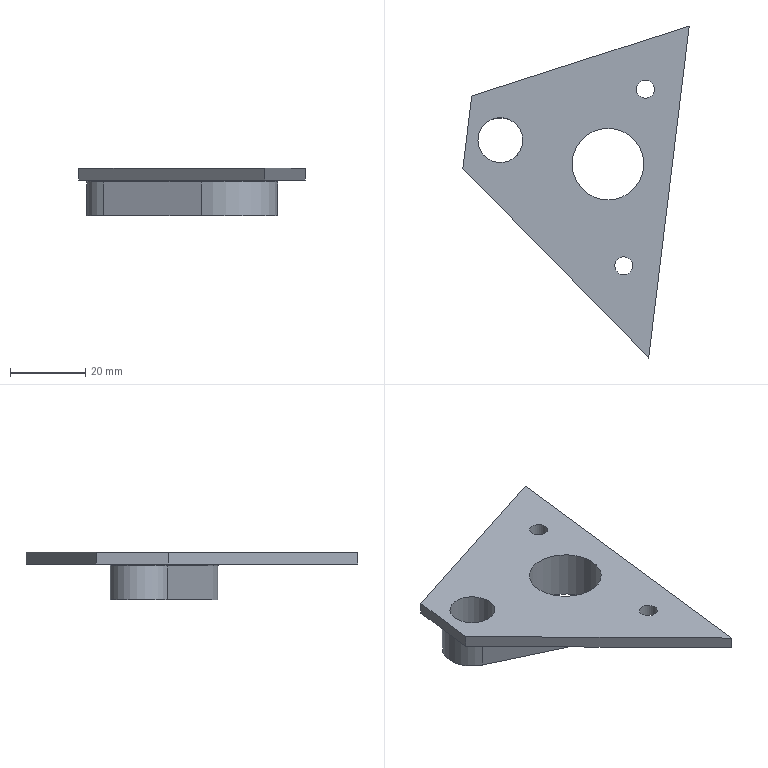Part | NX | features MG0301 nose pivot 24(left) 2 | 1 solid | 19 faces | box 60.073 x 88.114 x 12.7 mm | volume 14652 mm3 | plane 9 | cylinder 8 | torus 2 | commonest cylinder face diameters 1.016 x2 4.763 x2 11.906 x1 15.875 x1 19.05 x1 28.575 x1
STEP:
#1=CARTESIAN_POINT('',(-317.5,-112.204,-9.525));
#2=VERTEX_POINT('',#1);
#3=CARTESIAN_POINT('',(-346.075,-112.204,-9.525));
#4=VERTEX_POINT('',#3);
#5=CARTESIAN_POINT('',(-353.678,-112.204,-9.525));
#6=DIRECTION('',(-1.,0.,0.));
#7=VECTOR('',#6,1000.);
#8=LINE('',#5,#7);
#9=EDGE_CURVE('',#2,#4,#8,.T.);
#10=ORIENTED_EDGE('',*,*,#9,.T.);
#11=CARTESIAN_POINT('',(-349.652,-128.301,-9.525));
#12=VERTEX_POINT('',#11);
#13=CARTESIAN_POINT('',(-346.075,-120.65,-9.525));
#14=DIRECTION('',(0.,0.,1.));
#15=DIRECTION('',(1.,0.,0.));
#16=AXIS2_PLACEMENT_3D('',#13,#14,#15);
#17=CIRCLE('',#16,8.445);
#18=EDGE_CURVE('',#4,#12,#17,.T.);
#19=ORIENTED_EDGE('',*,*,#18,.T.);
#20=CARTESIAN_POINT('',(-323.766,-140.403,-9.525));
#21=VERTEX_POINT('',#20);
#22=CARTESIAN_POINT('',(-360.395,-123.278,-9.525));
#23=DIRECTION('',(0.9059,-0.4235,0.));
#24=VECTOR('',#23,1000.);
#25=LINE('',#22,#24);
#26=EDGE_CURVE('',#12,#21,#25,.T.);
#27=ORIENTED_EDGE('',*,*,#26,.T.);
#28=CARTESIAN_POINT('',(-317.5,-127.,-9.525));
#29=DIRECTION('',(0.,0.,1.));
#30=DIRECTION('',(1.,0.,0.));
#31=AXIS2_PLACEMENT_3D('',#28,#29,#30);
#32=CIRCLE('',#31,14.796);
#33=EDGE_CURVE('',#21,#2,#32,.T.);
#34=ORIENTED_EDGE('',*,*,#33,.T.);
#35=EDGE_LOOP('',(#10,#19,#27,#34));
#36=FACE_BOUND('',#35,.T.);
#37=CARTESIAN_POINT('',(-315.677,-153.957,-9.525));
#38=VERTEX_POINT('',#37);
#39=CARTESIAN_POINT('',(-313.296,-153.957,-9.525));
#40=DIRECTION('',(0.,0.,-1.));
#41=DIRECTION('',(-1.,0.,0.));
#42=AXIS2_PLACEMENT_3D('',#39,#40,#41);
#43=CIRCLE('',#42,2.381);
#44=EDGE_CURVE('',#38,#38,#43,.T.);
#45=ORIENTED_EDGE('',*,*,#44,.F.);
#46=EDGE_LOOP('',(#45));
#47=FACE_BOUND('',#46,.T.);
#48=CARTESIAN_POINT('',(-356.021,-128.145,-9.525));
#49=VERTEX_POINT('',#48);
#50=CARTESIAN_POINT('',(-353.678,-108.911,-9.525));
#51=VERTEX_POINT('',#50);
#52=CARTESIAN_POINT('',(-353.678,-108.911,-9.525));
#53=DIRECTION('',(0.1209,0.9927,0.));
#54=VECTOR('',#53,1000.);
#55=LINE('',#52,#54);
#56=EDGE_CURVE('',#49,#51,#55,.T.);
#57=ORIENTED_EDGE('',*,*,#56,.T.);
#58=CARTESIAN_POINT('',(-295.949,-90.332,-9.525));
#59=VERTEX_POINT('',#58);
#60=CARTESIAN_POINT('',(-353.678,-108.911,-9.525));
#61=DIRECTION('',(0.9519,0.3064,0.));
#62=VECTOR('',#61,1000.);
#63=LINE('',#60,#62);
#64=EDGE_CURVE('',#51,#59,#63,.T.);
#65=ORIENTED_EDGE('',*,*,#64,.T.);
#66=CARTESIAN_POINT('',(-306.684,-178.446,-9.525));
#67=VERTEX_POINT('',#66);
#68=CARTESIAN_POINT('',(-295.949,-90.332,-9.525));
#69=DIRECTION('',(-0.1209,-0.9927,0.));
#70=VECTOR('',#69,1000.);
#71=LINE('',#68,#70);
#72=EDGE_CURVE('',#59,#67,#71,.T.);
#73=ORIENTED_EDGE('',*,*,#72,.T.);
#74=CARTESIAN_POINT('',(-306.684,-178.446,-9.525));
#75=DIRECTION('',(-0.7002,0.7139,0.));
#76=VECTOR('',#75,1000.);
#77=LINE('',#74,#76);
#78=EDGE_CURVE('',#67,#49,#77,.T.);
#79=ORIENTED_EDGE('',*,*,#78,.T.);
#80=EDGE_LOOP('',(#57,#65,#73,#79));
#81=FACE_BOUND('',#80,.T.);
#82=CARTESIAN_POINT('',(-309.973,-107.134,-9.525));
#83=VERTEX_POINT('',#82);
#84=CARTESIAN_POINT('',(-307.591,-107.134,-9.525));
#85=DIRECTION('',(0.,0.,-1.));
#86=DIRECTION('',(-1.,0.,0.));
#87=AXIS2_PLACEMENT_3D('',#84,#85,#86);
#88=CIRCLE('',#87,2.381);
#89=EDGE_CURVE('',#83,#83,#88,.T.);
#90=ORIENTED_EDGE('',*,*,#89,.F.);
#91=EDGE_LOOP('',(#90));
#92=FACE_BOUND('',#91,.T.);
#93=CARTESIAN_POINT('',(-353.678,-108.911,-9.525));
#94=DIRECTION('',(0.,0.,1.));
#95=DIRECTION('',(1.,0.,0.));
#96=AXIS2_PLACEMENT_3D('',#93,#94,#95);
#97=PLANE('',#96);
#98=ADVANCED_FACE('',(#36,#47,#81,#92),#97,.F.);
#99=CARTESIAN_POINT('',(-340.122,-120.65,-6.35));
#100=VERTEX_POINT('',#99);
#101=CARTESIAN_POINT('',(-346.075,-120.65,-6.35));
#102=DIRECTION('',(0.,0.,1.));
#103=DIRECTION('',(1.,0.,0.));
#104=AXIS2_PLACEMENT_3D('',#101,#102,#103);
#105=CIRCLE('',#104,5.953);
#106=EDGE_CURVE('',#100,#100,#105,.T.);
#107=ORIENTED_EDGE('',*,*,#106,.F.);
#108=EDGE_LOOP('',(#107));
#109=FACE_BOUND('',#108,.T.);
#110=CARTESIAN_POINT('',(-307.975,-127.,-6.35));
#111=VERTEX_POINT('',#110);
#112=CARTESIAN_POINT('',(-317.5,-127.,-6.35));
#113=DIRECTION('',(0.,0.,1.));
#114=DIRECTION('',(1.,0.,0.));
#115=AXIS2_PLACEMENT_3D('',#112,#113,#114);
#116=CIRCLE('',#115,9.525);
#117=EDGE_CURVE('',#111,#111,#116,.T.);
#118=ORIENTED_EDGE('',*,*,#117,.F.);
#119=EDGE_LOOP('',(#118));
#120=FACE_BOUND('',#119,.T.);
#121=CARTESIAN_POINT('',(-315.677,-153.957,-6.35));
#122=VERTEX_POINT('',#121);
#123=CARTESIAN_POINT('',(-313.296,-153.957,-6.35));
#124=DIRECTION('',(0.,0.,-1.));
#125=DIRECTION('',(-1.,0.,0.));
#126=AXIS2_PLACEMENT_3D('',#123,#124,#125);
#127=CIRCLE('',#126,2.381);
#128=EDGE_CURVE('',#122,#122,#127,.T.);
#129=ORIENTED_EDGE('',*,*,#128,.T.);
#130=EDGE_LOOP('',(#129));
#131=FACE_BOUND('',#130,.T.);
#132=CARTESIAN_POINT('',(-356.021,-128.145,-6.35));
#133=VERTEX_POINT('',#132);
#134=CARTESIAN_POINT('',(-353.678,-108.911,-6.35));
#135=VERTEX_POINT('',#134);
#136=CARTESIAN_POINT('',(-353.678,-108.911,-6.35));
#137=DIRECTION('',(0.1209,0.9927,0.));
#138=VECTOR('',#137,1000.);
#139=LINE('',#136,#138);
#140=EDGE_CURVE('',#133,#135,#139,.T.);
#141=ORIENTED_EDGE('',*,*,#140,.F.);
#142=CARTESIAN_POINT('',(-306.684,-178.446,-6.35));
#143=VERTEX_POINT('',#142);
#144=CARTESIAN_POINT('',(-306.684,-178.446,-6.35));
#145=DIRECTION('',(-0.7002,0.7139,0.));
#146=VECTOR('',#145,1000.);
#147=LINE('',#144,#146);
#148=EDGE_CURVE('',#143,#133,#147,.T.);
#149=ORIENTED_EDGE('',*,*,#148,.F.);
#150=CARTESIAN_POINT('',(-295.949,-90.332,-6.35));
#151=VERTEX_POINT('',#150);
#152=CARTESIAN_POINT('',(-295.949,-90.332,-6.35));
#153=DIRECTION('',(-0.1209,-0.9927,0.));
#154=VECTOR('',#153,1000.);
#155=LINE('',#152,#154);
#156=EDGE_CURVE('',#151,#143,#155,.T.);
#157=ORIENTED_EDGE('',*,*,#156,.F.);
#158=CARTESIAN_POINT('',(-353.678,-108.911,-6.35));
#159=DIRECTION('',(0.9519,0.3064,0.));
#160=VECTOR('',#159,1000.);
#161=LINE('',#158,#160);
#162=EDGE_CURVE('',#135,#151,#161,.T.);
#163=ORIENTED_EDGE('',*,*,#162,.F.);
#164=EDGE_LOOP('',(#141,#149,#157,#163));
#165=FACE_BOUND('',#164,.T.);
#166=CARTESIAN_POINT('',(-309.973,-107.134,-6.35));
#167=VERTEX_POINT('',#166);
#168=CARTESIAN_POINT('',(-307.591,-107.134,-6.35));
#169=DIRECTION('',(0.,0.,-1.));
#170=DIRECTION('',(-1.,0.,0.));
#171=AXIS2_PLACEMENT_3D('',#168,#169,#170);
#172=CIRCLE('',#171,2.381);
#173=EDGE_CURVE('',#167,#167,#172,.T.);
#174=ORIENTED_EDGE('',*,*,#173,.T.);
#175=EDGE_LOOP('',(#174));
#176=FACE_BOUND('',#175,.T.);
#177=CARTESIAN_POINT('',(-353.678,-108.911,-6.35));
#178=DIRECTION('',(0.,0.,1.));
#179=DIRECTION('',(1.,0.,0.));
#180=AXIS2_PLACEMENT_3D('',#177,#178,#179);
#181=PLANE('',#180);
#182=ADVANCED_FACE('',(#109,#120,#131,#165,#176),#181,.T.);
#183=ORIENTED_EDGE('',*,*,#140,.T.);
#184=CARTESIAN_POINT('',(-353.678,-108.911,-9.525));
#185=DIRECTION('',(0.,0.,1.));
#186=VECTOR('',#185,1000.);
#187=LINE('',#184,#186);
#188=EDGE_CURVE('',#51,#135,#187,.T.);
#189=ORIENTED_EDGE('',*,*,#188,.F.);
#190=ORIENTED_EDGE('',*,*,#56,.F.);
#191=CARTESIAN_POINT('',(-356.021,-128.145,-9.525));
#192=DIRECTION('',(0.,0.,1.));
#193=VECTOR('',#192,1000.);
#194=LINE('',#191,#193);
#195=EDGE_CURVE('',#49,#133,#194,.T.);
#196=ORIENTED_EDGE('',*,*,#195,.T.);
#197=EDGE_LOOP('',(#183,#189,#190,#196));
#198=FACE_BOUND('',#197,.T.);
#199=CARTESIAN_POINT('',(-353.678,-108.911,-9.525));
#200=DIRECTION('',(0.9927,-0.1209,0.));
#201=DIRECTION('',(0.1209,0.9927,0.));
#202=AXIS2_PLACEMENT_3D('',#199,#200,#201);
#203=PLANE('',#202);
#204=ADVANCED_FACE('',(#198),#203,.F.);
#205=ORIENTED_EDGE('',*,*,#162,.T.);
#206=CARTESIAN_POINT('',(-295.949,-90.332,-9.525));
#207=DIRECTION('',(0.,0.,1.));
#208=VECTOR('',#207,1000.);
#209=LINE('',#206,#208);
#210=EDGE_CURVE('',#59,#151,#209,.T.);
#211=ORIENTED_EDGE('',*,*,#210,.F.);
#212=ORIENTED_EDGE('',*,*,#64,.F.);
#213=ORIENTED_EDGE('',*,*,#188,.T.);
#214=EDGE_LOOP('',(#205,#211,#212,#213));
#215=FACE_BOUND('',#214,.T.);
#216=CARTESIAN_POINT('',(-353.678,-108.911,-9.525));
#217=DIRECTION('',(0.3064,-0.9519,0.));
#218=DIRECTION('',(0.9519,0.3064,0.));
#219=AXIS2_PLACEMENT_3D('',#216,#217,#218);
#220=PLANE('',#219);
#221=ADVANCED_FACE('',(#215),#220,.F.);
#222=ORIENTED_EDGE('',*,*,#156,.T.);
#223=CARTESIAN_POINT('',(-306.684,-178.446,-9.525));
#224=DIRECTION('',(0.,0.,1.));
#225=VECTOR('',#224,1000.);
#226=LINE('',#223,#225);
#227=EDGE_CURVE('',#67,#143,#226,.T.);
#228=ORIENTED_EDGE('',*,*,#227,.F.);
#229=ORIENTED_EDGE('',*,*,#72,.F.);
#230=ORIENTED_EDGE('',*,*,#210,.T.);
#231=EDGE_LOOP('',(#222,#228,#229,#230));
#232=FACE_BOUND('',#231,.T.);
#233=CARTESIAN_POINT('',(-295.949,-90.332,-9.525));
#234=DIRECTION('',(-0.9927,0.1209,0.));
#235=DIRECTION('',(-0.1209,-0.9927,0.));
#236=AXIS2_PLACEMENT_3D('',#233,#234,#235);
#237=PLANE('',#236);
#238=ADVANCED_FACE('',(#232),#237,.F.);
#239=ORIENTED_EDGE('',*,*,#148,.T.);
#240=ORIENTED_EDGE('',*,*,#195,.F.);
#241=ORIENTED_EDGE('',*,*,#78,.F.);
#242=ORIENTED_EDGE('',*,*,#227,.T.);
#243=EDGE_LOOP('',(#239,#240,#241,#242));
#244=FACE_BOUND('',#243,.T.);
#245=CARTESIAN_POINT('',(-306.684,-178.446,-9.525));
#246=DIRECTION('',(0.7139,0.7002,0.));
#247=DIRECTION('',(-0.7002,0.7139,0.));
#248=AXIS2_PLACEMENT_3D('',#245,#246,#247);
#249=PLANE('',#248);
#250=ADVANCED_FACE('',(#244),#249,.F.);
#251=ORIENTED_EDGE('',*,*,#44,.T.);
#252=EDGE_LOOP('',(#251));
#253=FACE_BOUND('',#252,.T.);
#254=ORIENTED_EDGE('',*,*,#128,.F.);
#255=EDGE_LOOP('',(#254));
#256=FACE_BOUND('',#255,.T.);
#257=CARTESIAN_POINT('',(-313.296,-153.957,-9.525));
#258=DIRECTION('',(0.,0.,1.));
#259=DIRECTION('',(1.,0.,0.));
#260=AXIS2_PLACEMENT_3D('',#257,#258,#259);
#261=CYLINDRICAL_SURFACE('',#260,2.381);
#262=ADVANCED_FACE('',(#253,#256),#261,.F.);
#263=ORIENTED_EDGE('',*,*,#89,.T.);
#264=EDGE_LOOP('',(#263));
#265=FACE_BOUND('',#264,.T.);
#266=ORIENTED_EDGE('',*,*,#173,.F.);
#267=EDGE_LOOP('',(#266));
#268=FACE_BOUND('',#267,.T.);
#269=CARTESIAN_POINT('',(-307.591,-107.134,-9.525));
#270=DIRECTION('',(0.,0.,1.));
#271=DIRECTION('',(1.,0.,0.));
#272=AXIS2_PLACEMENT_3D('',#269,#270,#271);
#273=CYLINDRICAL_SURFACE('',#272,2.381);
#274=ADVANCED_FACE('',(#265,#268),#273,.F.);
#275=CARTESIAN_POINT('',(-349.437,-127.84,-19.05));
#276=VERTEX_POINT('',#275);
#277=CARTESIAN_POINT('',(-349.437,-127.84,-10.033));
#278=VERTEX_POINT('',#277);
#279=CARTESIAN_POINT('',(-349.437,-127.84,-19.05));
#280=DIRECTION('',(0.,0.,1.));
#281=VECTOR('',#280,1000.);
#282=LINE('',#279,#281);
#283=EDGE_CURVE('',#276,#278,#282,.T.);
#284=ORIENTED_EDGE('',*,*,#283,.T.);
#285=CARTESIAN_POINT('',(-346.075,-112.713,-10.033));
#286=VERTEX_POINT('',#285);
#287=CARTESIAN_POINT('',(-346.075,-120.65,-10.033));
#288=DIRECTION('',(0.,0.,1.));
#289=DIRECTION('',(1.,0.,0.));
#290=AXIS2_PLACEMENT_3D('',#287,#288,#289);
#291=CIRCLE('',#290,7.938);
#292=EDGE_CURVE('',#278,#286,#291,.F.);
#293=ORIENTED_EDGE('',*,*,#292,.T.);
#294=CARTESIAN_POINT('',(-346.075,-112.713,-19.05));
#295=VERTEX_POINT('',#294);
#296=CARTESIAN_POINT('',(-346.075,-112.713,-19.05));
#297=DIRECTION('',(0.,0.,1.));
#298=VECTOR('',#297,1000.);
#299=LINE('',#296,#298);
#300=EDGE_CURVE('',#295,#286,#299,.T.);
#301=ORIENTED_EDGE('',*,*,#300,.F.);
#302=CARTESIAN_POINT('',(-346.075,-120.65,-19.05));
#303=DIRECTION('',(0.,0.,1.));
#304=DIRECTION('',(1.,0.,0.));
#305=AXIS2_PLACEMENT_3D('',#302,#303,#304);
#306=CIRCLE('',#305,7.938);
#307=EDGE_CURVE('',#295,#276,#306,.T.);
#308=ORIENTED_EDGE('',*,*,#307,.T.);
#309=EDGE_LOOP('',(#284,#293,#301,#308));
#310=FACE_BOUND('',#309,.T.);
#311=CARTESIAN_POINT('',(-346.075,-120.65,-19.05));
#312=DIRECTION('',(0.,0.,1.));
#313=DIRECTION('',(1.,0.,0.));
#314=AXIS2_PLACEMENT_3D('',#311,#312,#313);
#315=CYLINDRICAL_SURFACE('',#314,7.938);
#316=ADVANCED_FACE('',(#310),#315,.T.);
#317=ORIENTED_EDGE('',*,*,#300,.T.);
#318=CARTESIAN_POINT('',(-317.5,-112.713,-10.033));
#319=VERTEX_POINT('',#318);
#320=CARTESIAN_POINT('',(-353.678,-112.713,-10.033));
#321=DIRECTION('',(-1.,0.,0.));
#322=VECTOR('',#321,1000.);
#323=LINE('',#320,#322);
#324=EDGE_CURVE('',#286,#319,#323,.F.);
#325=ORIENTED_EDGE('',*,*,#324,.T.);
#326=CARTESIAN_POINT('',(-317.5,-112.713,-19.05));
#327=VERTEX_POINT('',#326);
#328=CARTESIAN_POINT('',(-317.5,-112.713,-19.05));
#329=DIRECTION('',(0.,0.,1.));
#330=VECTOR('',#329,1000.);
#331=LINE('',#328,#330);
#332=EDGE_CURVE('',#327,#319,#331,.T.);
#333=ORIENTED_EDGE('',*,*,#332,.F.);
#334=CARTESIAN_POINT('',(-353.678,-112.713,-19.05));
#335=DIRECTION('',(-1.,0.,0.));
#336=VECTOR('',#335,1000.);
#337=LINE('',#334,#336);
#338=EDGE_CURVE('',#327,#295,#337,.T.);
#339=ORIENTED_EDGE('',*,*,#338,.T.);
#340=EDGE_LOOP('',(#317,#325,#333,#339));
#341=FACE_BOUND('',#340,.T.);
#342=CARTESIAN_POINT('',(-353.678,-112.713,-19.05));
#343=DIRECTION('',(0.,1.,0.));
#344=DIRECTION('',(0.,0.,1.));
#345=AXIS2_PLACEMENT_3D('',#342,#343,#344);
#346=PLANE('',#345);
#347=ADVANCED_FACE('',(#341),#346,.T.);
#348=ORIENTED_EDGE('',*,*,#332,.T.);
#349=CARTESIAN_POINT('',(-323.551,-139.943,-10.033));
#350=VERTEX_POINT('',#349);
#351=CARTESIAN_POINT('',(-317.5,-127.,-10.033));
#352=DIRECTION('',(0.,0.,1.));
#353=DIRECTION('',(1.,0.,0.));
#354=AXIS2_PLACEMENT_3D('',#351,#352,#353);
#355=CIRCLE('',#354,14.287);
#356=EDGE_CURVE('',#319,#350,#355,.F.);
#357=ORIENTED_EDGE('',*,*,#356,.T.);
#358=CARTESIAN_POINT('',(-323.551,-139.943,-19.05));
#359=VERTEX_POINT('',#358);
#360=CARTESIAN_POINT('',(-323.551,-139.943,-19.05));
#361=DIRECTION('',(0.,0.,1.));
#362=VECTOR('',#361,1000.);
#363=LINE('',#360,#362);
#364=EDGE_CURVE('',#359,#350,#363,.T.);
#365=ORIENTED_EDGE('',*,*,#364,.F.);
#366=CARTESIAN_POINT('',(-317.5,-127.,-19.05));
#367=DIRECTION('',(0.,0.,1.));
#368=DIRECTION('',(1.,0.,0.));
#369=AXIS2_PLACEMENT_3D('',#366,#367,#368);
#370=CIRCLE('',#369,14.287);
#371=EDGE_CURVE('',#359,#327,#370,.T.);
#372=ORIENTED_EDGE('',*,*,#371,.T.);
#373=EDGE_LOOP('',(#348,#357,#365,#372));
#374=FACE_BOUND('',#373,.T.);
#375=CARTESIAN_POINT('',(-317.5,-127.,-19.05));
#376=DIRECTION('',(0.,0.,1.));
#377=DIRECTION('',(1.,0.,0.));
#378=AXIS2_PLACEMENT_3D('',#375,#376,#377);
#379=CYLINDRICAL_SURFACE('',#378,14.287);
#380=ADVANCED_FACE('',(#374),#379,.T.);
#381=ORIENTED_EDGE('',*,*,#364,.T.);
#382=CARTESIAN_POINT('',(-360.18,-122.818,-10.033));
#383=DIRECTION('',(0.9059,-0.4235,0.));
#384=VECTOR('',#383,1000.);
#385=LINE('',#382,#384);
#386=EDGE_CURVE('',#350,#278,#385,.F.);
#387=ORIENTED_EDGE('',*,*,#386,.T.);
#388=ORIENTED_EDGE('',*,*,#283,.F.);
#389=CARTESIAN_POINT('',(-360.18,-122.818,-19.05));
#390=DIRECTION('',(0.9059,-0.4235,0.));
#391=VECTOR('',#390,1000.);
#392=LINE('',#389,#391);
#393=EDGE_CURVE('',#276,#359,#392,.T.);
#394=ORIENTED_EDGE('',*,*,#393,.T.);
#395=EDGE_LOOP('',(#381,#387,#388,#394));
#396=FACE_BOUND('',#395,.T.);
#397=CARTESIAN_POINT('',(-360.18,-122.818,-19.05));
#398=DIRECTION('',(-0.4235,-0.9059,0.));
#399=DIRECTION('',(0.9059,-0.4235,0.));
#400=AXIS2_PLACEMENT_3D('',#397,#398,#399);
#401=PLANE('',#400);
#402=ADVANCED_FACE('',(#396),#401,.T.);
#403=CARTESIAN_POINT('',(-340.122,-120.65,-19.05));
#404=VERTEX_POINT('',#403);
#405=CARTESIAN_POINT('',(-346.075,-120.65,-19.05));
#406=DIRECTION('',(0.,0.,1.));
#407=DIRECTION('',(1.,0.,0.));
#408=AXIS2_PLACEMENT_3D('',#405,#406,#407);
#409=CIRCLE('',#408,5.953);
#410=EDGE_CURVE('',#404,#404,#409,.T.);
#411=ORIENTED_EDGE('',*,*,#410,.T.);
#412=EDGE_LOOP('',(#411));
#413=FACE_BOUND('',#412,.T.);
#414=CARTESIAN_POINT('',(-307.975,-127.,-19.05));
#415=VERTEX_POINT('',#414);
#416=CARTESIAN_POINT('',(-317.5,-127.,-19.05));
#417=DIRECTION('',(0.,0.,1.));
#418=DIRECTION('',(1.,0.,0.));
#419=AXIS2_PLACEMENT_3D('',#416,#417,#418);
#420=CIRCLE('',#419,9.525);
#421=EDGE_CURVE('',#415,#415,#420,.T.);
#422=ORIENTED_EDGE('',*,*,#421,.T.);
#423=EDGE_LOOP('',(#422));
#424=FACE_BOUND('',#423,.T.);
#425=ORIENTED_EDGE('',*,*,#307,.F.);
#426=ORIENTED_EDGE('',*,*,#338,.F.);
#427=ORIENTED_EDGE('',*,*,#371,.F.);
#428=ORIENTED_EDGE('',*,*,#393,.F.);
#429=EDGE_LOOP('',(#425,#426,#427,#428));
#430=FACE_BOUND('',#429,.T.);
#431=CARTESIAN_POINT('',(-346.075,-120.65,-19.05));
#432=DIRECTION('',(0.,0.,1.));
#433=DIRECTION('',(1.,0.,0.));
#434=AXIS2_PLACEMENT_3D('',#431,#432,#433);
#435=PLANE('',#434);
#436=ADVANCED_FACE('',(#413,#424,#430),#435,.F.);
#437=ORIENTED_EDGE('',*,*,#421,.F.);
#438=EDGE_LOOP('',(#437));
#439=FACE_BOUND('',#438,.T.);
#440=ORIENTED_EDGE('',*,*,#117,.T.);
#441=EDGE_LOOP('',(#440));
#442=FACE_BOUND('',#441,.T.);
#443=CARTESIAN_POINT('',(-317.5,-127.,-19.05));
#444=DIRECTION('',(0.,0.,1.));
#445=DIRECTION('',(1.,0.,0.));
#446=AXIS2_PLACEMENT_3D('',#443,#444,#445);
#447=CYLINDRICAL_SURFACE('',#446,9.525);
#448=ADVANCED_FACE('',(#439,#442),#447,.F.);
#449=CARTESIAN_POINT('',(-323.766,-140.403,-10.033));
#450=DIRECTION('',(0.9059,-0.4235,0.));
#451=DIRECTION('',(0.4235,0.9059,0.));
#452=AXIS2_PLACEMENT_3D('',#449,#450,#451);
#453=CIRCLE('',#452,0.508);
#454=EDGE_CURVE('',#350,#21,#453,.T.);
#455=ORIENTED_EDGE('',*,*,#454,.F.);
#456=ORIENTED_EDGE('',*,*,#356,.F.);
#457=CARTESIAN_POINT('',(-317.5,-112.204,-10.033));
#458=DIRECTION('',(1.,0.,0.));
#459=DIRECTION('',(0.,0.,-1.));
#460=AXIS2_PLACEMENT_3D('',#457,#458,#459);
#461=CIRCLE('',#460,0.508);
#462=EDGE_CURVE('',#2,#319,#461,.T.);
#463=ORIENTED_EDGE('',*,*,#462,.F.);
#464=ORIENTED_EDGE('',*,*,#33,.F.);
#465=EDGE_LOOP('',(#455,#456,#463,#464));
#466=FACE_BOUND('',#465,.T.);
#467=CARTESIAN_POINT('',(-317.5,-127.,-10.033));
#468=DIRECTION('',(0.,0.,1.));
#469=DIRECTION('',(1.,0.,0.));
#470=AXIS2_PLACEMENT_3D('',#467,#468,#469);
#471=TOROIDAL_SURFACE('',#470,14.796,0.508);
#472=ADVANCED_FACE('',(#466),#471,.F.);
#473=ORIENTED_EDGE('',*,*,#462,.T.);
#474=ORIENTED_EDGE('',*,*,#324,.F.);
#475=CARTESIAN_POINT('',(-346.075,-112.204,-10.033));
#476=DIRECTION('',(1.,0.,0.));
#477=DIRECTION('',(0.,0.,-1.));
#478=AXIS2_PLACEMENT_3D('',#475,#476,#477);
#479=CIRCLE('',#478,0.508);
#480=EDGE_CURVE('',#4,#286,#479,.T.);
#481=ORIENTED_EDGE('',*,*,#480,.F.);
#482=ORIENTED_EDGE('',*,*,#9,.F.);
#483=EDGE_LOOP('',(#473,#474,#481,#482));
#484=FACE_BOUND('',#483,.T.);
#485=CARTESIAN_POINT('',(-353.678,-112.204,-10.033));
#486=DIRECTION('',(-1.,0.,0.));
#487=DIRECTION('',(0.,0.,1.));
#488=AXIS2_PLACEMENT_3D('',#485,#486,#487);
#489=CYLINDRICAL_SURFACE('',#488,0.508);
#490=ADVANCED_FACE('',(#484),#489,.F.);
#491=ORIENTED_EDGE('',*,*,#454,.T.);
#492=ORIENTED_EDGE('',*,*,#26,.F.);
#493=CARTESIAN_POINT('',(-349.652,-128.301,-10.033));
#494=DIRECTION('',(0.9059,-0.4235,0.));
#495=DIRECTION('',(0.4235,0.9059,0.));
#496=AXIS2_PLACEMENT_3D('',#493,#494,#495);
#497=CIRCLE('',#496,0.508);
#498=EDGE_CURVE('',#278,#12,#497,.T.);
#499=ORIENTED_EDGE('',*,*,#498,.F.);
#500=ORIENTED_EDGE('',*,*,#386,.F.);
#501=EDGE_LOOP('',(#491,#492,#499,#500));
#502=FACE_BOUND('',#501,.T.);
#503=CARTESIAN_POINT('',(-360.395,-123.278,-10.033));
#504=DIRECTION('',(0.9059,-0.4235,0.));
#505=DIRECTION('',(0.4235,0.9059,0.));
#506=AXIS2_PLACEMENT_3D('',#503,#504,#505);
#507=CYLINDRICAL_SURFACE('',#506,0.508);
#508=ADVANCED_FACE('',(#502),#507,.F.);
#509=ORIENTED_EDGE('',*,*,#480,.T.);
#510=ORIENTED_EDGE('',*,*,#292,.F.);
#511=ORIENTED_EDGE('',*,*,#498,.T.);
#512=ORIENTED_EDGE('',*,*,#18,.F.);
#513=EDGE_LOOP('',(#509,#510,#511,#512));
#514=FACE_BOUND('',#513,.T.);
#515=CARTESIAN_POINT('',(-346.075,-120.65,-10.033));
#516=DIRECTION('',(0.,0.,1.));
#517=DIRECTION('',(1.,0.,0.));
#518=AXIS2_PLACEMENT_3D('',#515,#516,#517);
#519=TOROIDAL_SURFACE('',#518,8.445,0.508);
#520=ADVANCED_FACE('',(#514),#519,.F.);
#521=ORIENTED_EDGE('',*,*,#106,.T.);
#522=EDGE_LOOP('',(#521));
#523=FACE_BOUND('',#522,.T.);
#524=ORIENTED_EDGE('',*,*,#410,.F.);
#525=EDGE_LOOP('',(#524));
#526=FACE_BOUND('',#525,.T.);
#527=CARTESIAN_POINT('',(-346.075,-120.65,-19.05));
#528=DIRECTION('',(0.,0.,1.));
#529=DIRECTION('',(1.,0.,0.));
#530=AXIS2_PLACEMENT_3D('',#527,#528,#529);
#531=CYLINDRICAL_SURFACE('',#530,5.953);
#532=ADVANCED_FACE('',(#523,#526),#531,.F.);
#533=CLOSED_SHELL('',(#98,#182,#204,#221,#238,#250,#262,#274,#316,#347,#380,#402,#436,#448,#472,#490,#508,#520,#532));
#534=MANIFOLD_SOLID_BREP('',#533);
#535=(LENGTH_UNIT()NAMED_UNIT(*)SI_UNIT(.MILLI.,.METRE.));
#536=UNCERTAINTY_MEASURE_WITH_UNIT(LENGTH_MEASURE(0.00001),#535,'','');
#537=(NAMED_UNIT(*)PLANE_ANGLE_UNIT()SI_UNIT($,.RADIAN.));
#538=(NAMED_UNIT(*)SI_UNIT($,.STERADIAN.)SOLID_ANGLE_UNIT());
#539=(GEOMETRIC_REPRESENTATION_CONTEXT(3)GLOBAL_UNCERTAINTY_ASSIGNED_CONTEXT((#536))GLOBAL_UNIT_ASSIGNED_CONTEXT((#535,#537,#538))REPRESENTATION_CONTEXT('',''));
#540=ADVANCED_BREP_SHAPE_REPRESENTATION('',(#534),#539);